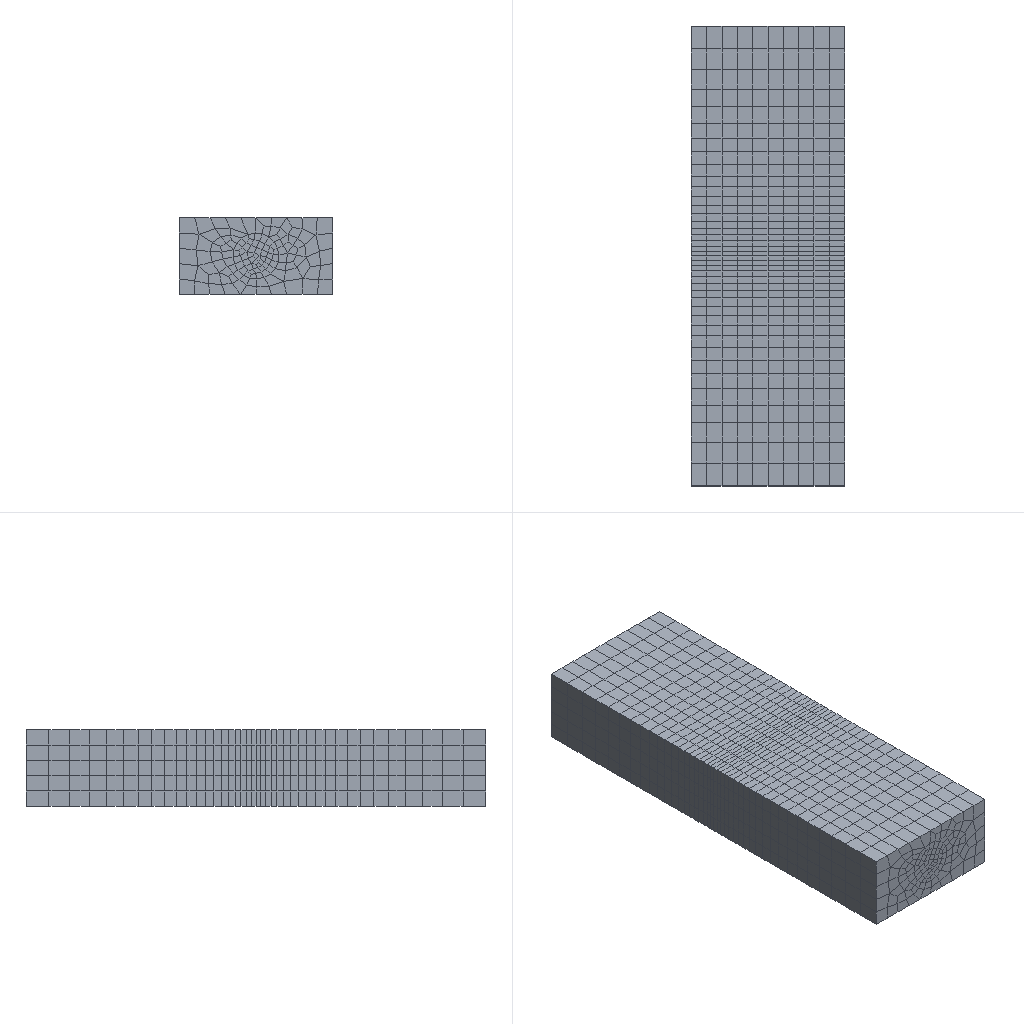Simulation study | abaqus
Set-up summary:
category,name,step,type,value,unit,region
solver,abaqus
solver,version,,,Abaqus/Standard 2020
units,not stated in the deck,,not stated
analysis,deck,,thermal,thermal
load_step,Step-1,Step-1,thermal
load_step,requested,,,1
mesh,nodes,,,6090
mesh,elements,,,5160
element_type,DC3D8,,solid,5160
load,load commands in deck,,count,3
bc,support commands in deck,,count,1
material,MATERIAL-1,,in results
check,setup vs results,,match,"per instance, exact: element labels, types and connectivity; labels of the nodes the elements use; coordinates of those nodes at SINGLE_PRECISION in 1 of 2 instance(s)"
Abaqus input file, long lists of numbers shortened:
*Heading
** Job name: Job-1 Model name: Model-1
** Generated by: Abaqus/CAE 2020
*Preprint, echo=NO, model=NO, history=NO, contact=NO
**
** PARTS
**
*Part, name=Part-1
*Node
      1,   5.832,         -15.,   1.252
      2,          10.,         -15.,           5.
** (3043 more lines like these left out)
*Element, type=DC3D8
   1,   12,   51,   81,   13,  157,  196,  226,  158
   2,   73,   52,   82,   81,  218,  197,  227,  226
** (2578 more lines like these left out)
*Nset, nset=Set-1, generate
    1,  3045,     1
*Elset, elset=Set-1, generate
    1,  2580,     1
** Section: Section-1
*Solid Section, elset=Set-1, material=Material-1
,
*End Part
**
**
** ASSEMBLY
**
*Assembly, name=Assembly
**
*Instance, name=Part-1-1, part=Part-1
         10.,         -15.,           0.
         10.,         -15.,           0.,          10.,         -15.,           1.,         180.
*End Instance
**
*Instance, name=Part-1-2, part=Part-1
          0.,          15.,           0.
*End Instance
**
*Nset, nset=Set-1, instance=Part-1-1, generate
    1,  3045,     1
*Nset, nset=Set-1, instance=Part-1-2, generate
    1,  3045,     1
*Elset, elset=Set-1, instance=Part-1-1, generate
    1,  2580,     1
*Elset, elset=Set-1, instance=Part-1-2, generate
    1,  2580,     1
*Elset, elset=_Surf-1_S1, internal, instance=Part-1-2, generate
  1,  48,   1
*Surface, type=ELEMENT, name=Surf-1
_Surf-1_S1, S1
*Elset, elset=_Surf-2_S1, internal, instance=Part-1-1, generate
  1,  48,   1
*Surface, type=ELEMENT, name=Surf-2
_Surf-2_S1, S1
*Elset, elset=_Surf-3_S1, internal, instance=Part-1-1, generate
   1,  129,    1
*Elset, elset=_Surf-3_S1, internal, instance=Part-1-2, generate
   1,  129,    1
*Elset, elset=_Surf-3_S6, internal, instance=Part-1-1
   66,   68,   71,   76,   79,   88,   91,  109,  110,  111,  112,  115,  195,  197,  200,  205
  208,  217,  220,  238,  239,  240,  241,  244,  324,  326,  329,  334,  337,  346,  349,  367
** (13 more lines like these left out)
*Elset, elset=_Surf-3_S6, internal, instance=Part-1-2
   66,   68,   71,   76,   79,   88,   91,  109,  110,  111,  112,  115,  195,  197,  200,  205
  208,  217,  220,  238,  239,  240,  241,  244,  324,  326,  329,  334,  337,  346,  349,  367
** (13 more lines like these left out)
*Elset, elset=_Surf-3_S5, internal, instance=Part-1-1
   57,   63,   67,   80,  125,  186,  192,  196,  209,  254,  315,  321,  325,  338,  383,  444
  450,  454,  467,  512,  573,  579,  583,  596,  641,  702,  708,  712,  725,  770,  831,  837
** (5 more lines like these left out)
*Elset, elset=_Surf-3_S5, internal, instance=Part-1-2
   57,   63,   67,   80,  125,  186,  192,  196,  209,  254,  315,  321,  325,  338,  383,  444
  450,  454,  467,  512,  573,  579,  583,  596,  641,  702,  708,  712,  725,  770,  831,  837
** (5 more lines like these left out)
*Elset, elset=_Surf-3_S4, internal, instance=Part-1-1
   67,   80,   99,  107,  108,  116,  117,  118,  126,  196,  209,  228,  236,  237,  245,  246
  247,  255,  325,  338,  357,  365,  366,  374,  375,  376,  384,  454,  467,  486,  494,  495
** (10 more lines like these left out)
*Elset, elset=_Surf-3_S4, internal, instance=Part-1-2
   67,   80,   99,  107,  108,  116,  117,  118,  126,  196,  209,  228,  236,  237,  245,  246
  247,  255,  325,  338,  357,  365,  366,  374,  375,  376,  384,  454,  467,  486,  494,  495
** (10 more lines like these left out)
*Elset, elset=_Surf-3_S2, internal, instance=Part-1-1, generate
 2452,  2580,     1
*Elset, elset=_Surf-3_S2, internal, instance=Part-1-2, generate
 2452,  2580,     1
*Elset, elset=_Surf-3_S3, internal, instance=Part-1-1
   49,   66,   76,   97,  178,  195,  205,  226,  307,  324,  334,  355,  436,  453,  463,  484
  565,  582,  592,  613,  694,  711,  721,  742,  823,  840,  850,  871,  952,  969,  979, 1000
** (3 more lines like these left out)
*Elset, elset=_Surf-3_S3, internal, instance=Part-1-2
   49,   66,   76,   97,  178,  195,  205,  226,  307,  324,  334,  355,  436,  453,  463,  484
  565,  582,  592,  613,  694,  711,  721,  742,  823,  840,  850,  871,  952,  969,  979, 1000
** (3 more lines like these left out)
*Surface, type=ELEMENT, name=Surf-3
_Surf-3_S1, S1
_Surf-3_S6, S6
_Surf-3_S4, S4
_Surf-3_S2, S2
_Surf-3_S5, S5
_Surf-3_S3, S3
*End Assembly
**
** MATERIALS
**
*Material, name=Material-1
*Conductivity
  6.475,  20.
   10.6, 250.
 13.369, 438.
    16., 623.
    20., 861.
    23.,1038.
    28.,1366.
   30.3,1554.
*Density
  4.7e-09,  20.
 4.67e-09, 318.
 4.61e-09, 765.
 4.59e-09, 985.
 4.55e-09,1227.
 4.43e-09,1616.
*Elastic
116000.,  0.45,   20.
111000., 0.445,  100.
105000., 0.438,  200.
102000.,  0.43,  300.
 99000., 0.427,  400.
 85000., 0.415,  500.
 72717., 0.398,  750.
 57392.,  0.38, 1000.
 38987.,  0.36, 1300.
*Expansion
 1e-05,
*Plastic, hardening=JOHNSON COOK
1100.,  590.,  0.41, 0.833, 1640.,   20.
*Rate Dependent, type=JOHNSON COOK
 0.0152,1.
*Specific Heat
 6.29e+08, 100.
 6.29e+08, 200.
 6.72e+08, 300.
  6.9e+08, 400.
 7.04e+08, 500.
 7.35e+08, 695.
 7.53e+08, 892.
 7.69e+08,1180.
 7.88e+08,1650.
**
** PHYSICAL CONSTANTS
**
*Physical Constants, absolute zero=-273., stefan boltzmann=5.67e-08
**
** PREDEFINED FIELDS
**
** Name: Predefined Field-1   Type: Temperature
*Initial Conditions, type=TEMPERATURE
Set-1, 20.
** ----------------------------------------------------------------
**
** STEP: Step-1
**
*Step, name=Step-1, nlgeom=NO, inc=10000
*Heat Transfer, end=PERIOD, deltmx=100000., mxdem=1.
0.1, 10., 0.0001, 10.,
**
** LOADS
**
** Name: Load-1   Type: Surface heat flux
*Dsflux
Surf-1, S, 1500.
** Name: Load-2   Type: Surface heat flux
*Dsflux
Surf-2, S, 1500.
**
** INTERACTIONS
**
** Interaction: Int-1
*Sfilm
Surf-3, F, 20., 0.01
**
** OUTPUT REQUESTS
**
*Restart, write, frequency=0
**
** FIELD OUTPUT: F-Output-1
**
*Output, field
*Node Output
NT, RFL
*Element Output, directions=YES
HFL, TEMP
*Output, history, frequency=0
*End Step
Results summary:
result,step,,partial,increments=0 time=0.0/10.0
result,analysis,,,"heat transfer, deltamx"
result,last_loadstep,,,1
result,primary field,,,NT11